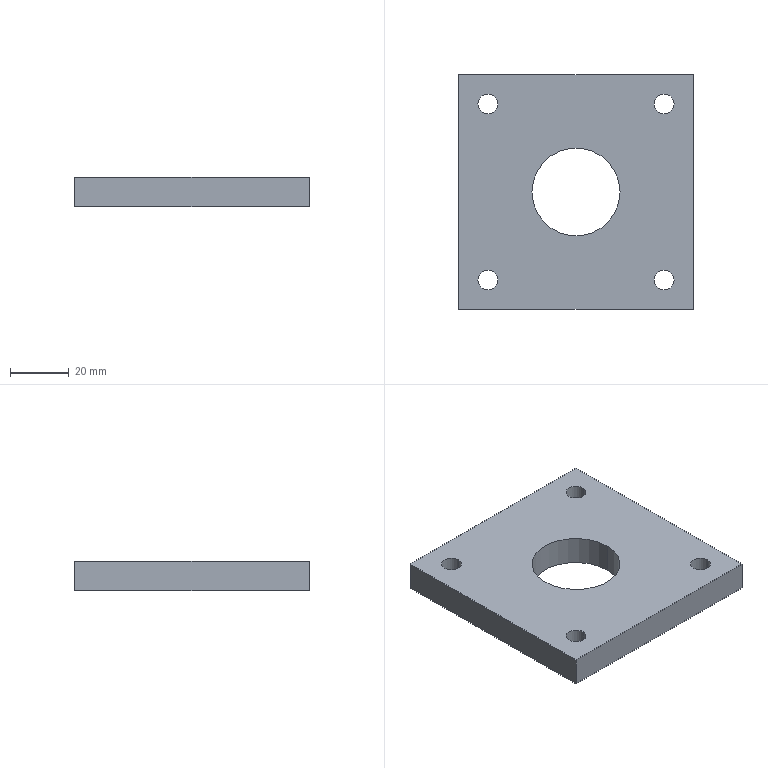Part | SolidWorks | features Extrusion 1, HoleWzd 1, ICE 1 | 1 solid | 16 faces | box 80 x 80 x 10 mm | volume 55479 mm3 | cylinder 10 | plane 6 | commonest cylinder face diameters 6.8 x8 30 x2
STEP:
#1=CARTESIAN_POINT('',(-15.,0.,0.));
#2=VERTEX_POINT('',#1);
#3=CARTESIAN_POINT('',(15.,0.,0.));
#4=VERTEX_POINT('',#3);
#5=CARTESIAN_POINT('',(0.,0.,0.));
#6=DIRECTION('',(0.,0.,1.));
#7=DIRECTION('',(1.,0.,0.));
#8=AXIS2_PLACEMENT_3D('',#5,#6,#7);
#9=CIRCLE('',#8,15.);
#10=EDGE_CURVE('',#2,#4,#9,.T.);
#11=ORIENTED_EDGE('',*,*,#10,.F.);
#12=CARTESIAN_POINT('',(-15.,0.,10.));
#13=VERTEX_POINT('',#12);
#14=CARTESIAN_POINT('',(-15.,0.,0.));
#15=DIRECTION('',(0.,0.,1.));
#16=VECTOR('',#15,1000.);
#17=LINE('',#14,#16);
#18=EDGE_CURVE('',#2,#13,#17,.T.);
#19=ORIENTED_EDGE('',*,*,#18,.T.);
#20=CARTESIAN_POINT('',(15.,0.,10.));
#21=VERTEX_POINT('',#20);
#22=CARTESIAN_POINT('',(0.,0.,10.));
#23=DIRECTION('',(0.,0.,1.));
#24=DIRECTION('',(1.,0.,0.));
#25=AXIS2_PLACEMENT_3D('',#22,#23,#24);
#26=CIRCLE('',#25,15.);
#27=EDGE_CURVE('',#13,#21,#26,.T.);
#28=ORIENTED_EDGE('',*,*,#27,.T.);
#29=CARTESIAN_POINT('',(15.,0.,0.));
#30=DIRECTION('',(0.,0.,1.));
#31=VECTOR('',#30,1000.);
#32=LINE('',#29,#31);
#33=EDGE_CURVE('',#4,#21,#32,.T.);
#34=ORIENTED_EDGE('',*,*,#33,.F.);
#35=EDGE_LOOP('',(#11,#19,#28,#34));
#36=FACE_OUTER_BOUND('',#35,.T.);
#37=CARTESIAN_POINT('',(0.,0.,0.));
#38=DIRECTION('',(0.,0.,1.));
#39=DIRECTION('',(1.,0.,0.));
#40=AXIS2_PLACEMENT_3D('',#37,#38,#39);
#41=CYLINDRICAL_SURFACE('',#40,15.);
#42=ADVANCED_FACE('',(#36),#41,.F.);
#43=CARTESIAN_POINT('',(-26.6,30.,0.));
#44=VERTEX_POINT('',#43);
#45=CARTESIAN_POINT('',(-33.4,30.,0.));
#46=VERTEX_POINT('',#45);
#47=CARTESIAN_POINT('',(-30.,30.,0.));
#48=DIRECTION('',(0.,0.,-1.));
#49=DIRECTION('',(-1.,0.,0.));
#50=AXIS2_PLACEMENT_3D('',#47,#48,#49);
#51=CIRCLE('',#50,3.4);
#52=EDGE_CURVE('',#44,#46,#51,.T.);
#53=ORIENTED_EDGE('',*,*,#52,.T.);
#54=CARTESIAN_POINT('',(-33.4,30.,10.));
#55=VERTEX_POINT('',#54);
#56=CARTESIAN_POINT('',(-33.4,30.,10.));
#57=DIRECTION('',(0.,0.,1.));
#58=VECTOR('',#57,1000.);
#59=LINE('',#56,#58);
#60=EDGE_CURVE('',#46,#55,#59,.T.);
#61=ORIENTED_EDGE('',*,*,#60,.T.);
#62=CARTESIAN_POINT('',(-26.6,30.,10.));
#63=VERTEX_POINT('',#62);
#64=CARTESIAN_POINT('',(-30.,30.,10.));
#65=DIRECTION('',(0.,0.,1.));
#66=DIRECTION('',(1.,0.,0.));
#67=AXIS2_PLACEMENT_3D('',#64,#65,#66);
#68=CIRCLE('',#67,3.4);
#69=EDGE_CURVE('',#55,#63,#68,.T.);
#70=ORIENTED_EDGE('',*,*,#69,.T.);
#71=CARTESIAN_POINT('',(-26.6,30.,10.));
#72=DIRECTION('',(0.,0.,1.));
#73=VECTOR('',#72,1000.);
#74=LINE('',#71,#73);
#75=EDGE_CURVE('',#44,#63,#74,.T.);
#76=ORIENTED_EDGE('',*,*,#75,.F.);
#77=EDGE_LOOP('',(#53,#61,#70,#76));
#78=FACE_OUTER_BOUND('',#77,.T.);
#79=CARTESIAN_POINT('',(-30.,30.,10.));
#80=DIRECTION('',(0.,0.,1.));
#81=DIRECTION('',(1.,0.,0.));
#82=AXIS2_PLACEMENT_3D('',#79,#80,#81);
#83=CYLINDRICAL_SURFACE('',#82,3.4);
#84=ADVANCED_FACE('',(#78),#83,.F.);
#85=CARTESIAN_POINT('',(33.4,30.,0.));
#86=VERTEX_POINT('',#85);
#87=CARTESIAN_POINT('',(26.6,30.,0.));
#88=VERTEX_POINT('',#87);
#89=CARTESIAN_POINT('',(30.,30.,0.));
#90=DIRECTION('',(0.,0.,-1.));
#91=DIRECTION('',(-1.,0.,0.));
#92=AXIS2_PLACEMENT_3D('',#89,#90,#91);
#93=CIRCLE('',#92,3.4);
#94=EDGE_CURVE('',#86,#88,#93,.T.);
#95=ORIENTED_EDGE('',*,*,#94,.T.);
#96=CARTESIAN_POINT('',(26.6,30.,10.));
#97=VERTEX_POINT('',#96);
#98=CARTESIAN_POINT('',(26.6,30.,10.));
#99=DIRECTION('',(0.,0.,1.));
#100=VECTOR('',#99,1000.);
#101=LINE('',#98,#100);
#102=EDGE_CURVE('',#88,#97,#101,.T.);
#103=ORIENTED_EDGE('',*,*,#102,.T.);
#104=CARTESIAN_POINT('',(33.4,30.,10.));
#105=VERTEX_POINT('',#104);
#106=CARTESIAN_POINT('',(30.,30.,10.));
#107=DIRECTION('',(0.,0.,1.));
#108=DIRECTION('',(1.,0.,0.));
#109=AXIS2_PLACEMENT_3D('',#106,#107,#108);
#110=CIRCLE('',#109,3.4);
#111=EDGE_CURVE('',#97,#105,#110,.T.);
#112=ORIENTED_EDGE('',*,*,#111,.T.);
#113=CARTESIAN_POINT('',(33.4,30.,10.));
#114=DIRECTION('',(0.,0.,1.));
#115=VECTOR('',#114,1000.);
#116=LINE('',#113,#115);
#117=EDGE_CURVE('',#86,#105,#116,.T.);
#118=ORIENTED_EDGE('',*,*,#117,.F.);
#119=EDGE_LOOP('',(#95,#103,#112,#118));
#120=FACE_OUTER_BOUND('',#119,.T.);
#121=CARTESIAN_POINT('',(30.,30.,10.));
#122=DIRECTION('',(0.,0.,1.));
#123=DIRECTION('',(1.,0.,0.));
#124=AXIS2_PLACEMENT_3D('',#121,#122,#123);
#125=CYLINDRICAL_SURFACE('',#124,3.4);
#126=ADVANCED_FACE('',(#120),#125,.F.);
#127=CARTESIAN_POINT('',(33.4,-30.,0.));
#128=VERTEX_POINT('',#127);
#129=CARTESIAN_POINT('',(26.6,-30.,0.));
#130=VERTEX_POINT('',#129);
#131=CARTESIAN_POINT('',(30.,-30.,0.));
#132=DIRECTION('',(0.,0.,-1.));
#133=DIRECTION('',(-1.,0.,0.));
#134=AXIS2_PLACEMENT_3D('',#131,#132,#133);
#135=CIRCLE('',#134,3.4);
#136=EDGE_CURVE('',#128,#130,#135,.T.);
#137=ORIENTED_EDGE('',*,*,#136,.T.);
#138=CARTESIAN_POINT('',(26.6,-30.,10.));
#139=VERTEX_POINT('',#138);
#140=CARTESIAN_POINT('',(26.6,-30.,10.));
#141=DIRECTION('',(0.,0.,1.));
#142=VECTOR('',#141,1000.);
#143=LINE('',#140,#142);
#144=EDGE_CURVE('',#130,#139,#143,.T.);
#145=ORIENTED_EDGE('',*,*,#144,.T.);
#146=CARTESIAN_POINT('',(33.4,-30.,10.));
#147=VERTEX_POINT('',#146);
#148=CARTESIAN_POINT('',(30.,-30.,10.));
#149=DIRECTION('',(0.,0.,1.));
#150=DIRECTION('',(1.,0.,0.));
#151=AXIS2_PLACEMENT_3D('',#148,#149,#150);
#152=CIRCLE('',#151,3.4);
#153=EDGE_CURVE('',#139,#147,#152,.T.);
#154=ORIENTED_EDGE('',*,*,#153,.T.);
#155=CARTESIAN_POINT('',(33.4,-30.,10.));
#156=DIRECTION('',(0.,0.,1.));
#157=VECTOR('',#156,1000.);
#158=LINE('',#155,#157);
#159=EDGE_CURVE('',#128,#147,#158,.T.);
#160=ORIENTED_EDGE('',*,*,#159,.F.);
#161=EDGE_LOOP('',(#137,#145,#154,#160));
#162=FACE_OUTER_BOUND('',#161,.T.);
#163=CARTESIAN_POINT('',(30.,-30.,10.));
#164=DIRECTION('',(0.,0.,1.));
#165=DIRECTION('',(1.,0.,0.));
#166=AXIS2_PLACEMENT_3D('',#163,#164,#165);
#167=CYLINDRICAL_SURFACE('',#166,3.4);
#168=ADVANCED_FACE('',(#162),#167,.F.);
#169=CARTESIAN_POINT('',(-26.6,-30.,0.));
#170=VERTEX_POINT('',#169);
#171=CARTESIAN_POINT('',(-33.4,-30.,0.));
#172=VERTEX_POINT('',#171);
#173=CARTESIAN_POINT('',(-30.,-30.,0.));
#174=DIRECTION('',(0.,0.,-1.));
#175=DIRECTION('',(-1.,0.,0.));
#176=AXIS2_PLACEMENT_3D('',#173,#174,#175);
#177=CIRCLE('',#176,3.4);
#178=EDGE_CURVE('',#170,#172,#177,.T.);
#179=ORIENTED_EDGE('',*,*,#178,.T.);
#180=CARTESIAN_POINT('',(-33.4,-30.,10.));
#181=VERTEX_POINT('',#180);
#182=CARTESIAN_POINT('',(-33.4,-30.,10.));
#183=DIRECTION('',(0.,0.,1.));
#184=VECTOR('',#183,1000.);
#185=LINE('',#182,#184);
#186=EDGE_CURVE('',#172,#181,#185,.T.);
#187=ORIENTED_EDGE('',*,*,#186,.T.);
#188=CARTESIAN_POINT('',(-26.6,-30.,10.));
#189=VERTEX_POINT('',#188);
#190=CARTESIAN_POINT('',(-30.,-30.,10.));
#191=DIRECTION('',(0.,0.,1.));
#192=DIRECTION('',(1.,0.,0.));
#193=AXIS2_PLACEMENT_3D('',#190,#191,#192);
#194=CIRCLE('',#193,3.4);
#195=EDGE_CURVE('',#181,#189,#194,.T.);
#196=ORIENTED_EDGE('',*,*,#195,.T.);
#197=CARTESIAN_POINT('',(-26.6,-30.,10.));
#198=DIRECTION('',(0.,0.,1.));
#199=VECTOR('',#198,1000.);
#200=LINE('',#197,#199);
#201=EDGE_CURVE('',#170,#189,#200,.T.);
#202=ORIENTED_EDGE('',*,*,#201,.F.);
#203=EDGE_LOOP('',(#179,#187,#196,#202));
#204=FACE_OUTER_BOUND('',#203,.T.);
#205=CARTESIAN_POINT('',(-30.,-30.,10.));
#206=DIRECTION('',(0.,0.,1.));
#207=DIRECTION('',(1.,0.,0.));
#208=AXIS2_PLACEMENT_3D('',#205,#206,#207);
#209=CYLINDRICAL_SURFACE('',#208,3.4);
#210=ADVANCED_FACE('',(#204),#209,.F.);
#211=CARTESIAN_POINT('',(-40.,40.,0.));
#212=VERTEX_POINT('',#211);
#213=CARTESIAN_POINT('',(-40.,-40.,0.));
#214=VERTEX_POINT('',#213);
#215=CARTESIAN_POINT('',(-40.,40.,0.));
#216=DIRECTION('',(0.,-1.,0.));
#217=VECTOR('',#216,1000.);
#218=LINE('',#215,#217);
#219=EDGE_CURVE('',#212,#214,#218,.T.);
#220=ORIENTED_EDGE('',*,*,#219,.T.);
#221=CARTESIAN_POINT('',(-40.,-40.,10.));
#222=VERTEX_POINT('',#221);
#223=CARTESIAN_POINT('',(-40.,-40.,10.));
#224=DIRECTION('',(0.,0.,-1.));
#225=VECTOR('',#224,1000.);
#226=LINE('',#223,#225);
#227=EDGE_CURVE('',#222,#214,#226,.T.);
#228=ORIENTED_EDGE('',*,*,#227,.F.);
#229=CARTESIAN_POINT('',(-40.,40.,10.));
#230=VERTEX_POINT('',#229);
#231=CARTESIAN_POINT('',(-40.,40.,10.));
#232=DIRECTION('',(0.,-1.,0.));
#233=VECTOR('',#232,1000.);
#234=LINE('',#231,#233);
#235=EDGE_CURVE('',#230,#222,#234,.T.);
#236=ORIENTED_EDGE('',*,*,#235,.F.);
#237=CARTESIAN_POINT('',(-40.,40.,10.));
#238=DIRECTION('',(0.,0.,-1.));
#239=VECTOR('',#238,1000.);
#240=LINE('',#237,#239);
#241=EDGE_CURVE('',#230,#212,#240,.T.);
#242=ORIENTED_EDGE('',*,*,#241,.T.);
#243=EDGE_LOOP('',(#220,#228,#236,#242));
#244=FACE_OUTER_BOUND('',#243,.T.);
#245=CARTESIAN_POINT('',(-40.,40.,10.));
#246=DIRECTION('',(1.,0.,0.));
#247=DIRECTION('',(0.,1.,0.));
#248=AXIS2_PLACEMENT_3D('',#245,#246,#247);
#249=PLANE('',#248);
#250=ADVANCED_FACE('',(#244),#249,.F.);
#251=CARTESIAN_POINT('',(40.,-40.,0.));
#252=VERTEX_POINT('',#251);
#253=CARTESIAN_POINT('',(40.,-40.,0.));
#254=DIRECTION('',(1.,0.,0.));
#255=VECTOR('',#254,1000.);
#256=LINE('',#253,#255);
#257=EDGE_CURVE('',#214,#252,#256,.T.);
#258=ORIENTED_EDGE('',*,*,#257,.T.);
#259=CARTESIAN_POINT('',(40.,-40.,10.));
#260=VERTEX_POINT('',#259);
#261=CARTESIAN_POINT('',(40.,-40.,10.));
#262=DIRECTION('',(0.,0.,-1.));
#263=VECTOR('',#262,1000.);
#264=LINE('',#261,#263);
#265=EDGE_CURVE('',#260,#252,#264,.T.);
#266=ORIENTED_EDGE('',*,*,#265,.F.);
#267=CARTESIAN_POINT('',(40.,-40.,10.));
#268=DIRECTION('',(1.,0.,0.));
#269=VECTOR('',#268,1000.);
#270=LINE('',#267,#269);
#271=EDGE_CURVE('',#222,#260,#270,.T.);
#272=ORIENTED_EDGE('',*,*,#271,.F.);
#273=ORIENTED_EDGE('',*,*,#227,.T.);
#274=EDGE_LOOP('',(#258,#266,#272,#273));
#275=FACE_OUTER_BOUND('',#274,.T.);
#276=CARTESIAN_POINT('',(40.,-40.,10.));
#277=DIRECTION('',(0.,1.,0.));
#278=DIRECTION('',(-1.,0.,0.));
#279=AXIS2_PLACEMENT_3D('',#276,#277,#278);
#280=PLANE('',#279);
#281=ADVANCED_FACE('',(#275),#280,.F.);
#282=CARTESIAN_POINT('',(40.,40.,0.));
#283=VERTEX_POINT('',#282);
#284=CARTESIAN_POINT('',(40.,40.,0.));
#285=DIRECTION('',(0.,1.,0.));
#286=VECTOR('',#285,1000.);
#287=LINE('',#284,#286);
#288=EDGE_CURVE('',#252,#283,#287,.T.);
#289=ORIENTED_EDGE('',*,*,#288,.T.);
#290=CARTESIAN_POINT('',(40.,40.,10.));
#291=VERTEX_POINT('',#290);
#292=CARTESIAN_POINT('',(40.,40.,10.));
#293=DIRECTION('',(0.,0.,-1.));
#294=VECTOR('',#293,1000.);
#295=LINE('',#292,#294);
#296=EDGE_CURVE('',#291,#283,#295,.T.);
#297=ORIENTED_EDGE('',*,*,#296,.F.);
#298=CARTESIAN_POINT('',(40.,40.,10.));
#299=DIRECTION('',(0.,1.,0.));
#300=VECTOR('',#299,1000.);
#301=LINE('',#298,#300);
#302=EDGE_CURVE('',#260,#291,#301,.T.);
#303=ORIENTED_EDGE('',*,*,#302,.F.);
#304=ORIENTED_EDGE('',*,*,#265,.T.);
#305=EDGE_LOOP('',(#289,#297,#303,#304));
#306=FACE_OUTER_BOUND('',#305,.T.);
#307=CARTESIAN_POINT('',(40.,40.,10.));
#308=DIRECTION('',(-1.,0.,0.));
#309=DIRECTION('',(0.,-1.,0.));
#310=AXIS2_PLACEMENT_3D('',#307,#308,#309);
#311=PLANE('',#310);
#312=ADVANCED_FACE('',(#306),#311,.F.);
#313=CARTESIAN_POINT('',(40.,40.,0.));
#314=DIRECTION('',(-1.,0.,0.));
#315=VECTOR('',#314,1000.);
#316=LINE('',#313,#315);
#317=EDGE_CURVE('',#283,#212,#316,.T.);
#318=ORIENTED_EDGE('',*,*,#317,.T.);
#319=ORIENTED_EDGE('',*,*,#241,.F.);
#320=CARTESIAN_POINT('',(40.,40.,10.));
#321=DIRECTION('',(-1.,0.,0.));
#322=VECTOR('',#321,1000.);
#323=LINE('',#320,#322);
#324=EDGE_CURVE('',#291,#230,#323,.T.);
#325=ORIENTED_EDGE('',*,*,#324,.F.);
#326=ORIENTED_EDGE('',*,*,#296,.T.);
#327=EDGE_LOOP('',(#318,#319,#325,#326));
#328=FACE_OUTER_BOUND('',#327,.T.);
#329=CARTESIAN_POINT('',(40.,40.,10.));
#330=DIRECTION('',(0.,-1.,0.));
#331=DIRECTION('',(1.,0.,0.));
#332=AXIS2_PLACEMENT_3D('',#329,#330,#331);
#333=PLANE('',#332);
#334=ADVANCED_FACE('',(#328),#333,.F.);
#335=CARTESIAN_POINT('',(0.,0.,10.));
#336=DIRECTION('',(0.,0.,1.));
#337=DIRECTION('',(1.,0.,0.));
#338=AXIS2_PLACEMENT_3D('',#335,#336,#337);
#339=CIRCLE('',#338,15.);
#340=EDGE_CURVE('',#21,#13,#339,.T.);
#341=ORIENTED_EDGE('',*,*,#340,.F.);
#342=ORIENTED_EDGE('',*,*,#27,.F.);
#343=EDGE_LOOP('',(#341,#342));
#344=FACE_BOUND('',#343,.T.);
#345=CARTESIAN_POINT('',(-30.,30.,10.));
#346=DIRECTION('',(0.,0.,1.));
#347=DIRECTION('',(1.,0.,0.));
#348=AXIS2_PLACEMENT_3D('',#345,#346,#347);
#349=CIRCLE('',#348,3.4);
#350=EDGE_CURVE('',#63,#55,#349,.T.);
#351=ORIENTED_EDGE('',*,*,#350,.F.);
#352=ORIENTED_EDGE('',*,*,#69,.F.);
#353=EDGE_LOOP('',(#351,#352));
#354=FACE_BOUND('',#353,.T.);
#355=CARTESIAN_POINT('',(30.,30.,10.));
#356=DIRECTION('',(0.,0.,1.));
#357=DIRECTION('',(1.,0.,0.));
#358=AXIS2_PLACEMENT_3D('',#355,#356,#357);
#359=CIRCLE('',#358,3.4);
#360=EDGE_CURVE('',#105,#97,#359,.T.);
#361=ORIENTED_EDGE('',*,*,#360,.F.);
#362=ORIENTED_EDGE('',*,*,#111,.F.);
#363=EDGE_LOOP('',(#361,#362));
#364=FACE_BOUND('',#363,.T.);
#365=CARTESIAN_POINT('',(30.,-30.,10.));
#366=DIRECTION('',(0.,0.,1.));
#367=DIRECTION('',(1.,0.,0.));
#368=AXIS2_PLACEMENT_3D('',#365,#366,#367);
#369=CIRCLE('',#368,3.4);
#370=EDGE_CURVE('',#147,#139,#369,.T.);
#371=ORIENTED_EDGE('',*,*,#370,.F.);
#372=ORIENTED_EDGE('',*,*,#153,.F.);
#373=EDGE_LOOP('',(#371,#372));
#374=FACE_BOUND('',#373,.T.);
#375=CARTESIAN_POINT('',(-30.,-30.,10.));
#376=DIRECTION('',(0.,0.,1.));
#377=DIRECTION('',(1.,0.,0.));
#378=AXIS2_PLACEMENT_3D('',#375,#376,#377);
#379=CIRCLE('',#378,3.4);
#380=EDGE_CURVE('',#189,#181,#379,.T.);
#381=ORIENTED_EDGE('',*,*,#380,.F.);
#382=ORIENTED_EDGE('',*,*,#195,.F.);
#383=EDGE_LOOP('',(#381,#382));
#384=FACE_BOUND('',#383,.T.);
#385=ORIENTED_EDGE('',*,*,#235,.T.);
#386=ORIENTED_EDGE('',*,*,#271,.T.);
#387=ORIENTED_EDGE('',*,*,#302,.T.);
#388=ORIENTED_EDGE('',*,*,#324,.T.);
#389=EDGE_LOOP('',(#385,#386,#387,#388));
#390=FACE_OUTER_BOUND('',#389,.T.);
#391=CARTESIAN_POINT('',(0.,0.,10.));
#392=DIRECTION('',(0.,0.,-1.));
#393=DIRECTION('',(-1.,0.,0.));
#394=AXIS2_PLACEMENT_3D('',#391,#392,#393);
#395=PLANE('',#394);
#396=ADVANCED_FACE('',(#344,#354,#364,#374,#384,#390),#395,.F.);
#397=CARTESIAN_POINT('',(0.,0.,0.));
#398=DIRECTION('',(0.,0.,1.));
#399=DIRECTION('',(1.,0.,0.));
#400=AXIS2_PLACEMENT_3D('',#397,#398,#399);
#401=CIRCLE('',#400,15.);
#402=EDGE_CURVE('',#4,#2,#401,.T.);
#403=ORIENTED_EDGE('',*,*,#402,.T.);
#404=ORIENTED_EDGE('',*,*,#10,.T.);
#405=EDGE_LOOP('',(#403,#404));
#406=FACE_BOUND('',#405,.T.);
#407=ORIENTED_EDGE('',*,*,#52,.F.);
#408=CARTESIAN_POINT('',(-30.,30.,0.));
#409=DIRECTION('',(0.,0.,-1.));
#410=DIRECTION('',(-1.,0.,0.));
#411=AXIS2_PLACEMENT_3D('',#408,#409,#410);
#412=CIRCLE('',#411,3.4);
#413=EDGE_CURVE('',#46,#44,#412,.T.);
#414=ORIENTED_EDGE('',*,*,#413,.F.);
#415=EDGE_LOOP('',(#407,#414));
#416=FACE_BOUND('',#415,.T.);
#417=ORIENTED_EDGE('',*,*,#94,.F.);
#418=CARTESIAN_POINT('',(30.,30.,0.));
#419=DIRECTION('',(0.,0.,-1.));
#420=DIRECTION('',(-1.,0.,0.));
#421=AXIS2_PLACEMENT_3D('',#418,#419,#420);
#422=CIRCLE('',#421,3.4);
#423=EDGE_CURVE('',#88,#86,#422,.T.);
#424=ORIENTED_EDGE('',*,*,#423,.F.);
#425=EDGE_LOOP('',(#417,#424));
#426=FACE_BOUND('',#425,.T.);
#427=ORIENTED_EDGE('',*,*,#136,.F.);
#428=CARTESIAN_POINT('',(30.,-30.,0.));
#429=DIRECTION('',(0.,0.,-1.));
#430=DIRECTION('',(-1.,0.,0.));
#431=AXIS2_PLACEMENT_3D('',#428,#429,#430);
#432=CIRCLE('',#431,3.4);
#433=EDGE_CURVE('',#130,#128,#432,.T.);
#434=ORIENTED_EDGE('',*,*,#433,.F.);
#435=EDGE_LOOP('',(#427,#434));
#436=FACE_BOUND('',#435,.T.);
#437=ORIENTED_EDGE('',*,*,#178,.F.);
#438=CARTESIAN_POINT('',(-30.,-30.,0.));
#439=DIRECTION('',(0.,0.,-1.));
#440=DIRECTION('',(-1.,0.,0.));
#441=AXIS2_PLACEMENT_3D('',#438,#439,#440);
#442=CIRCLE('',#441,3.4);
#443=EDGE_CURVE('',#172,#170,#442,.T.);
#444=ORIENTED_EDGE('',*,*,#443,.F.);
#445=EDGE_LOOP('',(#437,#444));
#446=FACE_BOUND('',#445,.T.);
#447=ORIENTED_EDGE('',*,*,#219,.F.);
#448=ORIENTED_EDGE('',*,*,#317,.F.);
#449=ORIENTED_EDGE('',*,*,#288,.F.);
#450=ORIENTED_EDGE('',*,*,#257,.F.);
#451=EDGE_LOOP('',(#447,#448,#449,#450));
#452=FACE_OUTER_BOUND('',#451,.T.);
#453=CARTESIAN_POINT('',(0.,0.,0.));
#454=DIRECTION('',(0.,0.,-1.));
#455=DIRECTION('',(-1.,0.,0.));
#456=AXIS2_PLACEMENT_3D('',#453,#454,#455);
#457=PLANE('',#456);
#458=ADVANCED_FACE('',(#406,#416,#426,#436,#446,#452),#457,.T.);
#459=ORIENTED_EDGE('',*,*,#186,.F.);
#460=ORIENTED_EDGE('',*,*,#443,.T.);
#461=ORIENTED_EDGE('',*,*,#201,.T.);
#462=ORIENTED_EDGE('',*,*,#380,.T.);
#463=EDGE_LOOP('',(#459,#460,#461,#462));
#464=FACE_OUTER_BOUND('',#463,.T.);
#465=CARTESIAN_POINT('',(-30.,-30.,10.));
#466=DIRECTION('',(0.,0.,1.));
#467=DIRECTION('',(1.,0.,0.));
#468=AXIS2_PLACEMENT_3D('',#465,#466,#467);
#469=CYLINDRICAL_SURFACE('',#468,3.4);
#470=ADVANCED_FACE('',(#464),#469,.F.);
#471=ORIENTED_EDGE('',*,*,#144,.F.);
#472=ORIENTED_EDGE('',*,*,#433,.T.);
#473=ORIENTED_EDGE('',*,*,#159,.T.);
#474=ORIENTED_EDGE('',*,*,#370,.T.);
#475=EDGE_LOOP('',(#471,#472,#473,#474));
#476=FACE_OUTER_BOUND('',#475,.T.);
#477=CARTESIAN_POINT('',(30.,-30.,10.));
#478=DIRECTION('',(0.,0.,1.));
#479=DIRECTION('',(1.,0.,0.));
#480=AXIS2_PLACEMENT_3D('',#477,#478,#479);
#481=CYLINDRICAL_SURFACE('',#480,3.4);
#482=ADVANCED_FACE('',(#476),#481,.F.);
#483=ORIENTED_EDGE('',*,*,#102,.F.);
#484=ORIENTED_EDGE('',*,*,#423,.T.);
#485=ORIENTED_EDGE('',*,*,#117,.T.);
#486=ORIENTED_EDGE('',*,*,#360,.T.);
#487=EDGE_LOOP('',(#483,#484,#485,#486));
#488=FACE_OUTER_BOUND('',#487,.T.);
#489=CARTESIAN_POINT('',(30.,30.,10.));
#490=DIRECTION('',(0.,0.,1.));
#491=DIRECTION('',(1.,0.,0.));
#492=AXIS2_PLACEMENT_3D('',#489,#490,#491);
#493=CYLINDRICAL_SURFACE('',#492,3.4);
#494=ADVANCED_FACE('',(#488),#493,.F.);
#495=ORIENTED_EDGE('',*,*,#60,.F.);
#496=ORIENTED_EDGE('',*,*,#413,.T.);
#497=ORIENTED_EDGE('',*,*,#75,.T.);
#498=ORIENTED_EDGE('',*,*,#350,.T.);
#499=EDGE_LOOP('',(#495,#496,#497,#498));
#500=FACE_OUTER_BOUND('',#499,.T.);
#501=CARTESIAN_POINT('',(-30.,30.,10.));
#502=DIRECTION('',(0.,0.,1.));
#503=DIRECTION('',(1.,0.,0.));
#504=AXIS2_PLACEMENT_3D('',#501,#502,#503);
#505=CYLINDRICAL_SURFACE('',#504,3.4);
#506=ADVANCED_FACE('',(#500),#505,.F.);
#507=ORIENTED_EDGE('',*,*,#18,.F.);
#508=ORIENTED_EDGE('',*,*,#402,.F.);
#509=ORIENTED_EDGE('',*,*,#33,.T.);
#510=ORIENTED_EDGE('',*,*,#340,.T.);
#511=EDGE_LOOP('',(#507,#508,#509,#510));
#512=FACE_OUTER_BOUND('',#511,.T.);
#513=CARTESIAN_POINT('',(0.,0.,0.));
#514=DIRECTION('',(0.,0.,1.));
#515=DIRECTION('',(1.,0.,0.));
#516=AXIS2_PLACEMENT_3D('',#513,#514,#515);
#517=CYLINDRICAL_SURFACE('',#516,15.);
#518=ADVANCED_FACE('',(#512),#517,.F.);
#519=CLOSED_SHELL('',(#42,#84,#126,#168,#210,#250,#281,#312,#334,#396,#458,#470,#482,#494,#506,#518));
#520=MANIFOLD_SOLID_BREP('',#519);
#521=CARTESIAN_POINT('',(0.,0.,0.));
#522=DIRECTION('',(0.,0.,1.));
#523=DIRECTION('',(1.,0.,0.));
#524=AXIS2_PLACEMENT_3D('',#521,#522,#523);
#525=(LENGTH_UNIT()NAMED_UNIT(*)SI_UNIT(.MILLI.,.METRE.));
#526=UNCERTAINTY_MEASURE_WITH_UNIT(LENGTH_MEASURE(0.00001),#525,'','');
#527=(NAMED_UNIT(*)PLANE_ANGLE_UNIT()SI_UNIT($,.RADIAN.));
#528=(NAMED_UNIT(*)SI_UNIT($,.STERADIAN.)SOLID_ANGLE_UNIT());
#529=(GEOMETRIC_REPRESENTATION_CONTEXT(3)GLOBAL_UNCERTAINTY_ASSIGNED_CONTEXT((#526))GLOBAL_UNIT_ASSIGNED_CONTEXT((#525,#527,#528))REPRESENTATION_CONTEXT('',''));
#530=ADVANCED_BREP_SHAPE_REPRESENTATION('',(#520,#524),#529);